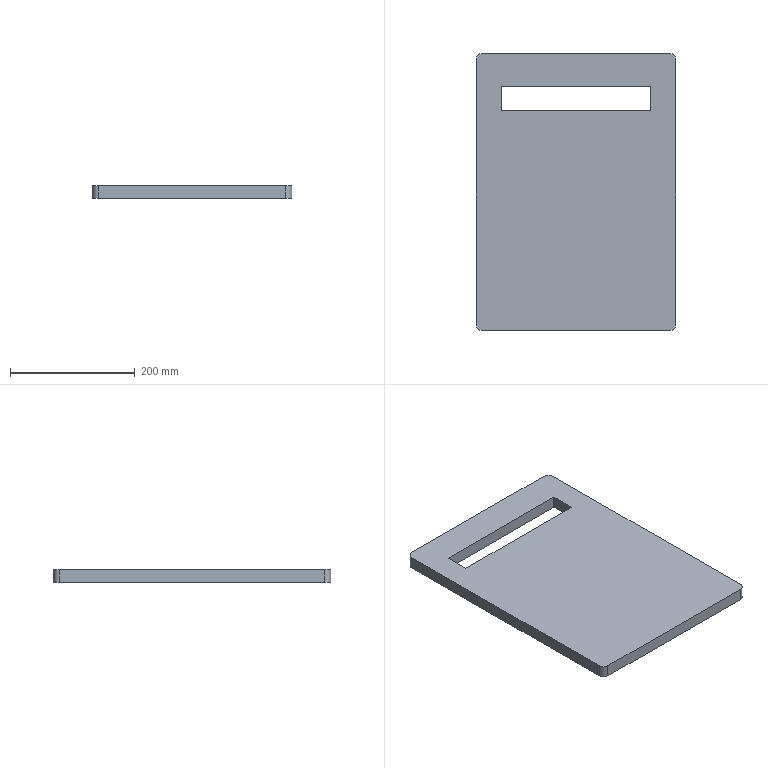Part | SolidWorks | features BaseBody 1 | 1 solid | 14 faces | box 320 x 445 x 20 mm | volume 2654283 mm3 | plane 10 | cylinder 4 | commonest cylinder face diameters 20 x4
STEP:
#1=CARTESIAN_POINT('',(-160.,-212.5,20.));
#2=VERTEX_POINT('',#1);
#3=CARTESIAN_POINT('',(-150.,-222.5,20.));
#4=VERTEX_POINT('',#3);
#5=CARTESIAN_POINT('',(-150.,-212.5,20.));
#6=DIRECTION('',(0.,0.,1.));
#7=DIRECTION('',(-1.,0.,0.));
#8=AXIS2_PLACEMENT_3D('',#5,#6,#7);
#9=CIRCLE('',#8,10.);
#10=EDGE_CURVE('',#2,#4,#9,.T.);
#11=ORIENTED_EDGE('',*,*,#10,.F.);
#12=CARTESIAN_POINT('',(-160.,-212.5,0.));
#13=VERTEX_POINT('',#12);
#14=CARTESIAN_POINT('',(-160.,-212.5,20.));
#15=DIRECTION('',(0.,0.,1.));
#16=VECTOR('',#15,1000.);
#17=LINE('',#14,#16);
#18=EDGE_CURVE('',#13,#2,#17,.T.);
#19=ORIENTED_EDGE('',*,*,#18,.F.);
#20=CARTESIAN_POINT('',(-150.,-222.5,0.));
#21=VERTEX_POINT('',#20);
#22=CARTESIAN_POINT('',(-150.,-212.5,0.));
#23=DIRECTION('',(0.,0.,-1.));
#24=DIRECTION('',(-1.,0.,0.));
#25=AXIS2_PLACEMENT_3D('',#22,#23,#24);
#26=CIRCLE('',#25,10.);
#27=EDGE_CURVE('',#21,#13,#26,.T.);
#28=ORIENTED_EDGE('',*,*,#27,.F.);
#29=CARTESIAN_POINT('',(-150.,-222.5,20.));
#30=DIRECTION('',(0.,0.,-1.));
#31=VECTOR('',#30,1000.);
#32=LINE('',#29,#31);
#33=EDGE_CURVE('',#4,#21,#32,.T.);
#34=ORIENTED_EDGE('',*,*,#33,.F.);
#35=EDGE_LOOP('',(#11,#19,#28,#34));
#36=FACE_OUTER_BOUND('',#35,.T.);
#37=CARTESIAN_POINT('',(-150.,-212.5,20.));
#38=DIRECTION('',(0.,0.,-1.));
#39=DIRECTION('',(-1.,0.,0.));
#40=AXIS2_PLACEMENT_3D('',#37,#38,#39);
#41=CYLINDRICAL_SURFACE('',#40,10.);
#42=ADVANCED_FACE('',(#36),#41,.T.);
#43=CARTESIAN_POINT('',(150.,-222.5,20.));
#44=VERTEX_POINT('',#43);
#45=CARTESIAN_POINT('',(160.,-212.5,20.));
#46=VERTEX_POINT('',#45);
#47=CARTESIAN_POINT('',(150.,-212.5,20.));
#48=DIRECTION('',(0.,0.,1.));
#49=DIRECTION('',(-1.,0.,0.));
#50=AXIS2_PLACEMENT_3D('',#47,#48,#49);
#51=CIRCLE('',#50,10.);
#52=EDGE_CURVE('',#44,#46,#51,.T.);
#53=ORIENTED_EDGE('',*,*,#52,.F.);
#54=CARTESIAN_POINT('',(150.,-222.5,0.));
#55=VERTEX_POINT('',#54);
#56=CARTESIAN_POINT('',(150.,-222.5,20.));
#57=DIRECTION('',(0.,0.,1.));
#58=VECTOR('',#57,1000.);
#59=LINE('',#56,#58);
#60=EDGE_CURVE('',#55,#44,#59,.T.);
#61=ORIENTED_EDGE('',*,*,#60,.F.);
#62=CARTESIAN_POINT('',(160.,-212.5,0.));
#63=VERTEX_POINT('',#62);
#64=CARTESIAN_POINT('',(150.,-212.5,0.));
#65=DIRECTION('',(0.,0.,-1.));
#66=DIRECTION('',(-1.,0.,0.));
#67=AXIS2_PLACEMENT_3D('',#64,#65,#66);
#68=CIRCLE('',#67,10.);
#69=EDGE_CURVE('',#63,#55,#68,.T.);
#70=ORIENTED_EDGE('',*,*,#69,.F.);
#71=CARTESIAN_POINT('',(160.,-212.5,20.));
#72=DIRECTION('',(0.,0.,-1.));
#73=VECTOR('',#72,1000.);
#74=LINE('',#71,#73);
#75=EDGE_CURVE('',#46,#63,#74,.T.);
#76=ORIENTED_EDGE('',*,*,#75,.F.);
#77=EDGE_LOOP('',(#53,#61,#70,#76));
#78=FACE_OUTER_BOUND('',#77,.T.);
#79=CARTESIAN_POINT('',(150.,-212.5,20.));
#80=DIRECTION('',(0.,0.,-1.));
#81=DIRECTION('',(-1.,0.,0.));
#82=AXIS2_PLACEMENT_3D('',#79,#80,#81);
#83=CYLINDRICAL_SURFACE('',#82,10.);
#84=ADVANCED_FACE('',(#78),#83,.T.);
#85=CARTESIAN_POINT('',(160.,212.5,20.));
#86=VERTEX_POINT('',#85);
#87=CARTESIAN_POINT('',(150.,222.5,20.));
#88=VERTEX_POINT('',#87);
#89=CARTESIAN_POINT('',(150.,212.5,20.));
#90=DIRECTION('',(0.,0.,1.));
#91=DIRECTION('',(-1.,0.,0.));
#92=AXIS2_PLACEMENT_3D('',#89,#90,#91);
#93=CIRCLE('',#92,10.);
#94=EDGE_CURVE('',#86,#88,#93,.T.);
#95=ORIENTED_EDGE('',*,*,#94,.F.);
#96=CARTESIAN_POINT('',(160.,212.5,0.));
#97=VERTEX_POINT('',#96);
#98=CARTESIAN_POINT('',(160.,212.5,20.));
#99=DIRECTION('',(0.,0.,1.));
#100=VECTOR('',#99,1000.);
#101=LINE('',#98,#100);
#102=EDGE_CURVE('',#97,#86,#101,.T.);
#103=ORIENTED_EDGE('',*,*,#102,.F.);
#104=CARTESIAN_POINT('',(150.,222.5,0.));
#105=VERTEX_POINT('',#104);
#106=CARTESIAN_POINT('',(150.,212.5,0.));
#107=DIRECTION('',(0.,0.,-1.));
#108=DIRECTION('',(-1.,0.,0.));
#109=AXIS2_PLACEMENT_3D('',#106,#107,#108);
#110=CIRCLE('',#109,10.);
#111=EDGE_CURVE('',#105,#97,#110,.T.);
#112=ORIENTED_EDGE('',*,*,#111,.F.);
#113=CARTESIAN_POINT('',(150.,222.5,20.));
#114=DIRECTION('',(0.,0.,-1.));
#115=VECTOR('',#114,1000.);
#116=LINE('',#113,#115);
#117=EDGE_CURVE('',#88,#105,#116,.T.);
#118=ORIENTED_EDGE('',*,*,#117,.F.);
#119=EDGE_LOOP('',(#95,#103,#112,#118));
#120=FACE_OUTER_BOUND('',#119,.T.);
#121=CARTESIAN_POINT('',(150.,212.5,20.));
#122=DIRECTION('',(0.,0.,-1.));
#123=DIRECTION('',(-1.,0.,0.));
#124=AXIS2_PLACEMENT_3D('',#121,#122,#123);
#125=CYLINDRICAL_SURFACE('',#124,10.);
#126=ADVANCED_FACE('',(#120),#125,.T.);
#127=CARTESIAN_POINT('',(-150.,222.5,20.));
#128=VERTEX_POINT('',#127);
#129=CARTESIAN_POINT('',(-160.,212.5,20.));
#130=VERTEX_POINT('',#129);
#131=CARTESIAN_POINT('',(-150.,212.5,20.));
#132=DIRECTION('',(0.,0.,1.));
#133=DIRECTION('',(-1.,0.,0.));
#134=AXIS2_PLACEMENT_3D('',#131,#132,#133);
#135=CIRCLE('',#134,10.);
#136=EDGE_CURVE('',#128,#130,#135,.T.);
#137=ORIENTED_EDGE('',*,*,#136,.F.);
#138=CARTESIAN_POINT('',(-150.,222.5,0.));
#139=VERTEX_POINT('',#138);
#140=CARTESIAN_POINT('',(-150.,222.5,20.));
#141=DIRECTION('',(0.,0.,1.));
#142=VECTOR('',#141,1000.);
#143=LINE('',#140,#142);
#144=EDGE_CURVE('',#139,#128,#143,.T.);
#145=ORIENTED_EDGE('',*,*,#144,.F.);
#146=CARTESIAN_POINT('',(-160.,212.5,0.));
#147=VERTEX_POINT('',#146);
#148=CARTESIAN_POINT('',(-150.,212.5,0.));
#149=DIRECTION('',(0.,0.,-1.));
#150=DIRECTION('',(-1.,0.,0.));
#151=AXIS2_PLACEMENT_3D('',#148,#149,#150);
#152=CIRCLE('',#151,10.);
#153=EDGE_CURVE('',#147,#139,#152,.T.);
#154=ORIENTED_EDGE('',*,*,#153,.F.);
#155=CARTESIAN_POINT('',(-160.,212.5,20.));
#156=DIRECTION('',(0.,0.,-1.));
#157=VECTOR('',#156,1000.);
#158=LINE('',#155,#157);
#159=EDGE_CURVE('',#130,#147,#158,.T.);
#160=ORIENTED_EDGE('',*,*,#159,.F.);
#161=EDGE_LOOP('',(#137,#145,#154,#160));
#162=FACE_OUTER_BOUND('',#161,.T.);
#163=CARTESIAN_POINT('',(-150.,212.5,20.));
#164=DIRECTION('',(0.,0.,-1.));
#165=DIRECTION('',(-1.,0.,0.));
#166=AXIS2_PLACEMENT_3D('',#163,#164,#165);
#167=CYLINDRICAL_SURFACE('',#166,10.);
#168=ADVANCED_FACE('',(#162),#167,.T.);
#169=CARTESIAN_POINT('',(120.,170.,20.));
#170=VERTEX_POINT('',#169);
#171=CARTESIAN_POINT('',(-120.,170.,20.));
#172=VERTEX_POINT('',#171);
#173=CARTESIAN_POINT('',(-120.,170.,20.));
#174=DIRECTION('',(-1.,0.,0.));
#175=VECTOR('',#174,1000.);
#176=LINE('',#173,#175);
#177=EDGE_CURVE('',#170,#172,#176,.T.);
#178=ORIENTED_EDGE('',*,*,#177,.T.);
#179=CARTESIAN_POINT('',(-120.,170.,0.));
#180=VERTEX_POINT('',#179);
#181=CARTESIAN_POINT('',(-120.,170.,0.));
#182=DIRECTION('',(0.,0.,1.));
#183=VECTOR('',#182,1000.);
#184=LINE('',#181,#183);
#185=EDGE_CURVE('',#180,#172,#184,.T.);
#186=ORIENTED_EDGE('',*,*,#185,.F.);
#187=CARTESIAN_POINT('',(120.,170.,0.));
#188=VERTEX_POINT('',#187);
#189=CARTESIAN_POINT('',(-120.,170.,0.));
#190=DIRECTION('',(-1.,0.,0.));
#191=VECTOR('',#190,1000.);
#192=LINE('',#189,#191);
#193=EDGE_CURVE('',#188,#180,#192,.T.);
#194=ORIENTED_EDGE('',*,*,#193,.F.);
#195=CARTESIAN_POINT('',(120.,170.,0.));
#196=DIRECTION('',(0.,0.,1.));
#197=VECTOR('',#196,1000.);
#198=LINE('',#195,#197);
#199=EDGE_CURVE('',#188,#170,#198,.T.);
#200=ORIENTED_EDGE('',*,*,#199,.T.);
#201=EDGE_LOOP('',(#178,#186,#194,#200));
#202=FACE_OUTER_BOUND('',#201,.T.);
#203=CARTESIAN_POINT('',(-120.,170.,0.));
#204=DIRECTION('',(0.,1.,0.));
#205=DIRECTION('',(1.,0.,0.));
#206=AXIS2_PLACEMENT_3D('',#203,#204,#205);
#207=PLANE('',#206);
#208=ADVANCED_FACE('',(#202),#207,.F.);
#209=CARTESIAN_POINT('',(-120.,130.,20.));
#210=VERTEX_POINT('',#209);
#211=CARTESIAN_POINT('',(-120.,130.,20.));
#212=DIRECTION('',(0.,-1.,0.));
#213=VECTOR('',#212,1000.);
#214=LINE('',#211,#213);
#215=EDGE_CURVE('',#172,#210,#214,.T.);
#216=ORIENTED_EDGE('',*,*,#215,.T.);
#217=CARTESIAN_POINT('',(-120.,130.,0.));
#218=VERTEX_POINT('',#217);
#219=CARTESIAN_POINT('',(-120.,130.,0.));
#220=DIRECTION('',(0.,0.,1.));
#221=VECTOR('',#220,1000.);
#222=LINE('',#219,#221);
#223=EDGE_CURVE('',#218,#210,#222,.T.);
#224=ORIENTED_EDGE('',*,*,#223,.F.);
#225=CARTESIAN_POINT('',(-120.,130.,0.));
#226=DIRECTION('',(0.,-1.,0.));
#227=VECTOR('',#226,1000.);
#228=LINE('',#225,#227);
#229=EDGE_CURVE('',#180,#218,#228,.T.);
#230=ORIENTED_EDGE('',*,*,#229,.F.);
#231=ORIENTED_EDGE('',*,*,#185,.T.);
#232=EDGE_LOOP('',(#216,#224,#230,#231));
#233=FACE_OUTER_BOUND('',#232,.T.);
#234=CARTESIAN_POINT('',(-120.,130.,0.));
#235=DIRECTION('',(-1.,0.,0.));
#236=DIRECTION('',(0.,0.,1.));
#237=AXIS2_PLACEMENT_3D('',#234,#235,#236);
#238=PLANE('',#237);
#239=ADVANCED_FACE('',(#233),#238,.F.);
#240=CARTESIAN_POINT('',(120.,130.,20.));
#241=VERTEX_POINT('',#240);
#242=CARTESIAN_POINT('',(-120.,130.,20.));
#243=DIRECTION('',(1.,0.,0.));
#244=VECTOR('',#243,1000.);
#245=LINE('',#242,#244);
#246=EDGE_CURVE('',#210,#241,#245,.T.);
#247=ORIENTED_EDGE('',*,*,#246,.T.);
#248=CARTESIAN_POINT('',(120.,130.,0.));
#249=VERTEX_POINT('',#248);
#250=CARTESIAN_POINT('',(120.,130.,0.));
#251=DIRECTION('',(0.,0.,1.));
#252=VECTOR('',#251,1000.);
#253=LINE('',#250,#252);
#254=EDGE_CURVE('',#249,#241,#253,.T.);
#255=ORIENTED_EDGE('',*,*,#254,.F.);
#256=CARTESIAN_POINT('',(-120.,130.,0.));
#257=DIRECTION('',(1.,0.,0.));
#258=VECTOR('',#257,1000.);
#259=LINE('',#256,#258);
#260=EDGE_CURVE('',#218,#249,#259,.T.);
#261=ORIENTED_EDGE('',*,*,#260,.F.);
#262=ORIENTED_EDGE('',*,*,#223,.T.);
#263=EDGE_LOOP('',(#247,#255,#261,#262));
#264=FACE_OUTER_BOUND('',#263,.T.);
#265=CARTESIAN_POINT('',(-120.,130.,0.));
#266=DIRECTION('',(0.,-1.,0.));
#267=DIRECTION('',(0.,0.,-1.));
#268=AXIS2_PLACEMENT_3D('',#265,#266,#267);
#269=PLANE('',#268);
#270=ADVANCED_FACE('',(#264),#269,.F.);
#271=CARTESIAN_POINT('',(120.,130.,20.));
#272=DIRECTION('',(0.,1.,0.));
#273=VECTOR('',#272,1000.);
#274=LINE('',#271,#273);
#275=EDGE_CURVE('',#241,#170,#274,.T.);
#276=ORIENTED_EDGE('',*,*,#275,.T.);
#277=ORIENTED_EDGE('',*,*,#199,.F.);
#278=CARTESIAN_POINT('',(120.,130.,0.));
#279=DIRECTION('',(0.,1.,0.));
#280=VECTOR('',#279,1000.);
#281=LINE('',#278,#280);
#282=EDGE_CURVE('',#249,#188,#281,.T.);
#283=ORIENTED_EDGE('',*,*,#282,.F.);
#284=ORIENTED_EDGE('',*,*,#254,.T.);
#285=EDGE_LOOP('',(#276,#277,#283,#284));
#286=FACE_OUTER_BOUND('',#285,.T.);
#287=CARTESIAN_POINT('',(120.,130.,0.));
#288=DIRECTION('',(1.,0.,0.));
#289=DIRECTION('',(0.,1.,0.));
#290=AXIS2_PLACEMENT_3D('',#287,#288,#289);
#291=PLANE('',#290);
#292=ADVANCED_FACE('',(#286),#291,.F.);
#293=ORIENTED_EDGE('',*,*,#282,.T.);
#294=ORIENTED_EDGE('',*,*,#193,.T.);
#295=ORIENTED_EDGE('',*,*,#229,.T.);
#296=ORIENTED_EDGE('',*,*,#260,.T.);
#297=EDGE_LOOP('',(#293,#294,#295,#296));
#298=FACE_BOUND('',#297,.T.);
#299=CARTESIAN_POINT('',(-160.,-222.5,0.));
#300=DIRECTION('',(0.,-1.,0.));
#301=VECTOR('',#300,1000.);
#302=LINE('',#299,#301);
#303=EDGE_CURVE('',#147,#13,#302,.T.);
#304=ORIENTED_EDGE('',*,*,#303,.F.);
#305=ORIENTED_EDGE('',*,*,#153,.T.);
#306=CARTESIAN_POINT('',(-160.,222.5,0.));
#307=DIRECTION('',(-1.,0.,0.));
#308=VECTOR('',#307,1000.);
#309=LINE('',#306,#308);
#310=EDGE_CURVE('',#105,#139,#309,.T.);
#311=ORIENTED_EDGE('',*,*,#310,.F.);
#312=ORIENTED_EDGE('',*,*,#111,.T.);
#313=CARTESIAN_POINT('',(160.,-222.5,0.));
#314=DIRECTION('',(0.,1.,0.));
#315=VECTOR('',#314,1000.);
#316=LINE('',#313,#315);
#317=EDGE_CURVE('',#63,#97,#316,.T.);
#318=ORIENTED_EDGE('',*,*,#317,.F.);
#319=ORIENTED_EDGE('',*,*,#69,.T.);
#320=CARTESIAN_POINT('',(-160.,-222.5,0.));
#321=DIRECTION('',(1.,0.,0.));
#322=VECTOR('',#321,1000.);
#323=LINE('',#320,#322);
#324=EDGE_CURVE('',#21,#55,#323,.T.);
#325=ORIENTED_EDGE('',*,*,#324,.F.);
#326=ORIENTED_EDGE('',*,*,#27,.T.);
#327=EDGE_LOOP('',(#304,#305,#311,#312,#318,#319,#325,#326));
#328=FACE_OUTER_BOUND('',#327,.T.);
#329=CARTESIAN_POINT('',(0.,0.,0.));
#330=DIRECTION('',(0.,0.,-1.));
#331=DIRECTION('',(0.,-1.,0.));
#332=AXIS2_PLACEMENT_3D('',#329,#330,#331);
#333=PLANE('',#332);
#334=ADVANCED_FACE('',(#298,#328),#333,.T.);
#335=ORIENTED_EDGE('',*,*,#177,.F.);
#336=ORIENTED_EDGE('',*,*,#275,.F.);
#337=ORIENTED_EDGE('',*,*,#246,.F.);
#338=ORIENTED_EDGE('',*,*,#215,.F.);
#339=EDGE_LOOP('',(#335,#336,#337,#338));
#340=FACE_BOUND('',#339,.T.);
#341=CARTESIAN_POINT('',(-160.,222.5,20.));
#342=DIRECTION('',(-1.,0.,0.));
#343=VECTOR('',#342,1000.);
#344=LINE('',#341,#343);
#345=EDGE_CURVE('',#88,#128,#344,.T.);
#346=ORIENTED_EDGE('',*,*,#345,.T.);
#347=ORIENTED_EDGE('',*,*,#136,.T.);
#348=CARTESIAN_POINT('',(-160.,-222.5,20.));
#349=DIRECTION('',(0.,-1.,0.));
#350=VECTOR('',#349,1000.);
#351=LINE('',#348,#350);
#352=EDGE_CURVE('',#130,#2,#351,.T.);
#353=ORIENTED_EDGE('',*,*,#352,.T.);
#354=ORIENTED_EDGE('',*,*,#10,.T.);
#355=CARTESIAN_POINT('',(-160.,-222.5,20.));
#356=DIRECTION('',(1.,0.,0.));
#357=VECTOR('',#356,1000.);
#358=LINE('',#355,#357);
#359=EDGE_CURVE('',#4,#44,#358,.T.);
#360=ORIENTED_EDGE('',*,*,#359,.T.);
#361=ORIENTED_EDGE('',*,*,#52,.T.);
#362=CARTESIAN_POINT('',(160.,-222.5,20.));
#363=DIRECTION('',(0.,1.,0.));
#364=VECTOR('',#363,1000.);
#365=LINE('',#362,#364);
#366=EDGE_CURVE('',#46,#86,#365,.T.);
#367=ORIENTED_EDGE('',*,*,#366,.T.);
#368=ORIENTED_EDGE('',*,*,#94,.T.);
#369=EDGE_LOOP('',(#346,#347,#353,#354,#360,#361,#367,#368));
#370=FACE_OUTER_BOUND('',#369,.T.);
#371=CARTESIAN_POINT('',(0.,0.,20.));
#372=DIRECTION('',(0.,0.,-1.));
#373=DIRECTION('',(0.,-1.,0.));
#374=AXIS2_PLACEMENT_3D('',#371,#372,#373);
#375=PLANE('',#374);
#376=ADVANCED_FACE('',(#340,#370),#375,.F.);
#377=ORIENTED_EDGE('',*,*,#324,.T.);
#378=ORIENTED_EDGE('',*,*,#60,.T.);
#379=ORIENTED_EDGE('',*,*,#359,.F.);
#380=ORIENTED_EDGE('',*,*,#33,.T.);
#381=EDGE_LOOP('',(#377,#378,#379,#380));
#382=FACE_OUTER_BOUND('',#381,.T.);
#383=CARTESIAN_POINT('',(-160.,-222.5,20.));
#384=DIRECTION('',(0.,1.,0.));
#385=DIRECTION('',(1.,0.,0.));
#386=AXIS2_PLACEMENT_3D('',#383,#384,#385);
#387=PLANE('',#386);
#388=ADVANCED_FACE('',(#382),#387,.F.);
#389=ORIENTED_EDGE('',*,*,#352,.F.);
#390=ORIENTED_EDGE('',*,*,#159,.T.);
#391=ORIENTED_EDGE('',*,*,#303,.T.);
#392=ORIENTED_EDGE('',*,*,#18,.T.);
#393=EDGE_LOOP('',(#389,#390,#391,#392));
#394=FACE_OUTER_BOUND('',#393,.T.);
#395=CARTESIAN_POINT('',(-160.,-222.5,20.));
#396=DIRECTION('',(1.,0.,0.));
#397=DIRECTION('',(0.,1.,0.));
#398=AXIS2_PLACEMENT_3D('',#395,#396,#397);
#399=PLANE('',#398);
#400=ADVANCED_FACE('',(#394),#399,.F.);
#401=ORIENTED_EDGE('',*,*,#310,.T.);
#402=ORIENTED_EDGE('',*,*,#144,.T.);
#403=ORIENTED_EDGE('',*,*,#345,.F.);
#404=ORIENTED_EDGE('',*,*,#117,.T.);
#405=EDGE_LOOP('',(#401,#402,#403,#404));
#406=FACE_OUTER_BOUND('',#405,.T.);
#407=CARTESIAN_POINT('',(-160.,222.5,20.));
#408=DIRECTION('',(0.,-1.,0.));
#409=DIRECTION('',(0.,0.,-1.));
#410=AXIS2_PLACEMENT_3D('',#407,#408,#409);
#411=PLANE('',#410);
#412=ADVANCED_FACE('',(#406),#411,.F.);
#413=ORIENTED_EDGE('',*,*,#317,.T.);
#414=ORIENTED_EDGE('',*,*,#102,.T.);
#415=ORIENTED_EDGE('',*,*,#366,.F.);
#416=ORIENTED_EDGE('',*,*,#75,.T.);
#417=EDGE_LOOP('',(#413,#414,#415,#416));
#418=FACE_OUTER_BOUND('',#417,.T.);
#419=CARTESIAN_POINT('',(160.,-222.5,20.));
#420=DIRECTION('',(-1.,0.,0.));
#421=DIRECTION('',(0.,0.,1.));
#422=AXIS2_PLACEMENT_3D('',#419,#420,#421);
#423=PLANE('',#422);
#424=ADVANCED_FACE('',(#418),#423,.F.);
#425=CLOSED_SHELL('',(#42,#84,#126,#168,#208,#239,#270,#292,#334,#376,#388,#400,#412,#424));
#426=MANIFOLD_SOLID_BREP('',#425);
#427=CARTESIAN_POINT('',(0.,0.,0.));
#428=DIRECTION('',(0.,0.,1.));
#429=DIRECTION('',(1.,0.,0.));
#430=AXIS2_PLACEMENT_3D('',#427,#428,#429);
#431=(LENGTH_UNIT()NAMED_UNIT(*)SI_UNIT(.MILLI.,.METRE.));
#432=UNCERTAINTY_MEASURE_WITH_UNIT(LENGTH_MEASURE(0.00001),#431,'','');
#433=(NAMED_UNIT(*)PLANE_ANGLE_UNIT()SI_UNIT($,.RADIAN.));
#434=(NAMED_UNIT(*)SI_UNIT($,.STERADIAN.)SOLID_ANGLE_UNIT());
#435=(GEOMETRIC_REPRESENTATION_CONTEXT(3)GLOBAL_UNCERTAINTY_ASSIGNED_CONTEXT((#432))GLOBAL_UNIT_ASSIGNED_CONTEXT((#431,#433,#434))REPRESENTATION_CONTEXT('',''));
#436=ADVANCED_BREP_SHAPE_REPRESENTATION('',(#426,#430),#435);